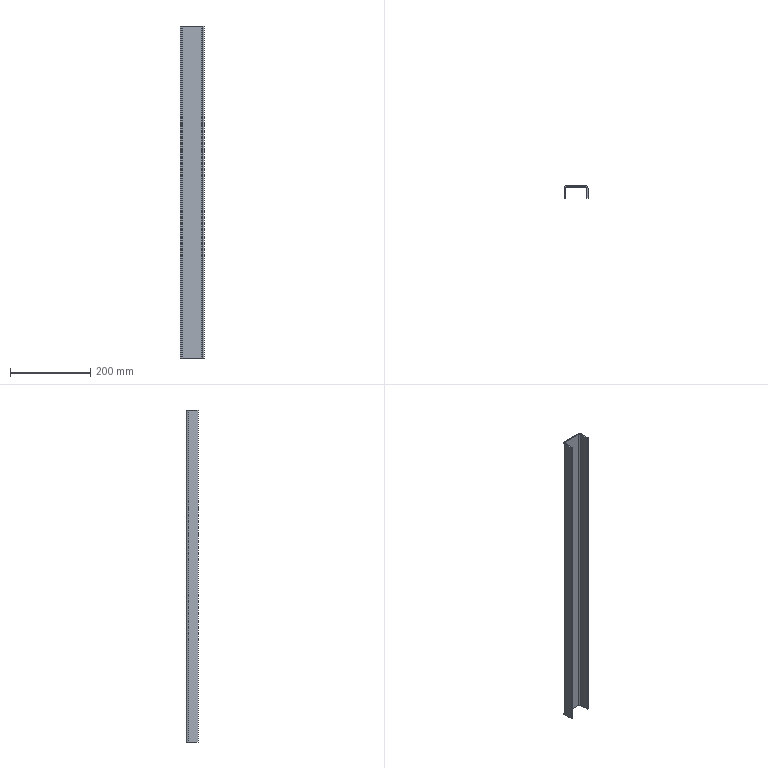Part | STEP file | VD-SYL0380DJ1006_1_1-13_VD-SYL0 | 1 solid | 14 faces | box 60 x 30 x 830 mm | volume 274242 mm3 | plane 10 | cylinder 4 | commonest cylinder face diameters 6 x2 12 x2
STEP:
#1=CARTESIAN_POINT('',(-24.,20.,415.));
#2=VERTEX_POINT('',#1);
#3=CARTESIAN_POINT('',(-24.,20.,-415.));
#4=VERTEX_POINT('',#3);
#5=CARTESIAN_POINT('',(-24.,20.,415.));
#6=DIRECTION('',(0.,0.,-1.));
#7=VECTOR('',#6,1000.);
#8=LINE('',#5,#7);
#9=EDGE_CURVE('',#2,#4,#8,.T.);
#10=ORIENTED_EDGE('',*,*,#9,.T.);
#11=CARTESIAN_POINT('',(-30.,14.,-415.));
#12=VERTEX_POINT('',#11);
#13=CARTESIAN_POINT('',(-24.,14.,-415.));
#14=DIRECTION('',(0.,0.,-1.));
#15=DIRECTION('',(-1.,0.,0.));
#16=AXIS2_PLACEMENT_3D('',#13,#14,#15);
#17=CIRCLE('',#16,6.);
#18=EDGE_CURVE('',#12,#4,#17,.T.);
#19=ORIENTED_EDGE('',*,*,#18,.F.);
#20=CARTESIAN_POINT('',(-30.,14.,415.));
#21=VERTEX_POINT('',#20);
#22=CARTESIAN_POINT('',(-30.,14.,-415.));
#23=DIRECTION('',(0.,0.,1.));
#24=VECTOR('',#23,1000.);
#25=LINE('',#22,#24);
#26=EDGE_CURVE('',#12,#21,#25,.T.);
#27=ORIENTED_EDGE('',*,*,#26,.T.);
#28=CARTESIAN_POINT('',(-24.,14.,415.));
#29=DIRECTION('',(0.,0.,1.));
#30=DIRECTION('',(0.,1.,0.));
#31=AXIS2_PLACEMENT_3D('',#28,#29,#30);
#32=CIRCLE('',#31,6.);
#33=EDGE_CURVE('',#2,#21,#32,.T.);
#34=ORIENTED_EDGE('',*,*,#33,.F.);
#35=EDGE_LOOP('',(#10,#19,#27,#34));
#36=FACE_OUTER_BOUND('',#35,.T.);
#37=CARTESIAN_POINT('',(-24.,14.,1496.988));
#38=DIRECTION('',(0.,0.,-1.));
#39=DIRECTION('',(-1.,0.,0.));
#40=AXIS2_PLACEMENT_3D('',#37,#38,#39);
#41=CYLINDRICAL_SURFACE('',#40,6.);
#42=ADVANCED_FACE('',(#36),#41,.T.);
#43=CARTESIAN_POINT('',(-30.,-10.,415.));
#44=VERTEX_POINT('',#43);
#45=CARTESIAN_POINT('',(-30.,-10.,-415.));
#46=VERTEX_POINT('',#45);
#47=CARTESIAN_POINT('',(-30.,-10.,415.));
#48=DIRECTION('',(0.,0.,-1.));
#49=VECTOR('',#48,1000.);
#50=LINE('',#47,#49);
#51=EDGE_CURVE('',#44,#46,#50,.T.);
#52=ORIENTED_EDGE('',*,*,#51,.T.);
#53=CARTESIAN_POINT('',(-27.,-10.,-415.));
#54=VERTEX_POINT('',#53);
#55=CARTESIAN_POINT('',(-27.,-10.,-415.));
#56=DIRECTION('',(-1.,0.,0.));
#57=VECTOR('',#56,1000.);
#58=LINE('',#55,#57);
#59=EDGE_CURVE('',#54,#46,#58,.T.);
#60=ORIENTED_EDGE('',*,*,#59,.F.);
#61=CARTESIAN_POINT('',(-27.,-10.,415.));
#62=VERTEX_POINT('',#61);
#63=CARTESIAN_POINT('',(-27.,-10.,415.));
#64=DIRECTION('',(0.,0.,-1.));
#65=VECTOR('',#64,1000.);
#66=LINE('',#63,#65);
#67=EDGE_CURVE('',#62,#54,#66,.T.);
#68=ORIENTED_EDGE('',*,*,#67,.F.);
#69=CARTESIAN_POINT('',(-30.,-10.,415.));
#70=DIRECTION('',(1.,0.,0.));
#71=VECTOR('',#70,1000.);
#72=LINE('',#69,#71);
#73=EDGE_CURVE('',#44,#62,#72,.T.);
#74=ORIENTED_EDGE('',*,*,#73,.F.);
#75=EDGE_LOOP('',(#52,#60,#68,#74));
#76=FACE_OUTER_BOUND('',#75,.T.);
#77=CARTESIAN_POINT('',(-28.5,-10.,0.));
#78=DIRECTION('',(0.,-1.,0.));
#79=DIRECTION('',(0.,0.,-1.));
#80=AXIS2_PLACEMENT_3D('',#77,#78,#79);
#81=PLANE('',#80);
#82=ADVANCED_FACE('',(#76),#81,.T.);
#83=CARTESIAN_POINT('',(-27.,14.,-415.));
#84=VERTEX_POINT('',#83);
#85=CARTESIAN_POINT('',(-27.,-10.,-415.));
#86=DIRECTION('',(0.,1.,0.));
#87=VECTOR('',#86,1000.);
#88=LINE('',#85,#87);
#89=EDGE_CURVE('',#54,#84,#88,.T.);
#90=ORIENTED_EDGE('',*,*,#89,.T.);
#91=CARTESIAN_POINT('',(-27.,14.,415.));
#92=VERTEX_POINT('',#91);
#93=CARTESIAN_POINT('',(-27.,14.,415.));
#94=DIRECTION('',(0.,0.,-1.));
#95=VECTOR('',#94,1000.);
#96=LINE('',#93,#95);
#97=EDGE_CURVE('',#92,#84,#96,.T.);
#98=ORIENTED_EDGE('',*,*,#97,.F.);
#99=CARTESIAN_POINT('',(-27.,-10.,415.));
#100=DIRECTION('',(0.,1.,0.));
#101=VECTOR('',#100,1000.);
#102=LINE('',#99,#101);
#103=EDGE_CURVE('',#62,#92,#102,.T.);
#104=ORIENTED_EDGE('',*,*,#103,.F.);
#105=ORIENTED_EDGE('',*,*,#67,.T.);
#106=EDGE_LOOP('',(#90,#98,#104,#105));
#107=FACE_OUTER_BOUND('',#106,.T.);
#108=CARTESIAN_POINT('',(-27.,20.,-415.));
#109=DIRECTION('',(-1.,0.,0.));
#110=DIRECTION('',(0.,0.,1.));
#111=AXIS2_PLACEMENT_3D('',#108,#109,#110);
#112=PLANE('',#111);
#113=ADVANCED_FACE('',(#107),#112,.F.);
#114=CARTESIAN_POINT('',(-24.,17.,-415.));
#115=VERTEX_POINT('',#114);
#116=CARTESIAN_POINT('',(-24.,14.,-415.));
#117=DIRECTION('',(0.,0.,1.));
#118=DIRECTION('',(0.,1.,0.));
#119=AXIS2_PLACEMENT_3D('',#116,#117,#118);
#120=CIRCLE('',#119,3.);
#121=EDGE_CURVE('',#115,#84,#120,.T.);
#122=ORIENTED_EDGE('',*,*,#121,.F.);
#123=CARTESIAN_POINT('',(-24.,17.,415.));
#124=VERTEX_POINT('',#123);
#125=CARTESIAN_POINT('',(-24.,17.,-415.));
#126=DIRECTION('',(0.,0.,1.));
#127=VECTOR('',#126,1000.);
#128=LINE('',#125,#127);
#129=EDGE_CURVE('',#115,#124,#128,.T.);
#130=ORIENTED_EDGE('',*,*,#129,.T.);
#131=CARTESIAN_POINT('',(-24.,14.,415.));
#132=DIRECTION('',(0.,0.,-1.));
#133=DIRECTION('',(-1.,0.,0.));
#134=AXIS2_PLACEMENT_3D('',#131,#132,#133);
#135=CIRCLE('',#134,3.);
#136=EDGE_CURVE('',#92,#124,#135,.T.);
#137=ORIENTED_EDGE('',*,*,#136,.F.);
#138=ORIENTED_EDGE('',*,*,#97,.T.);
#139=EDGE_LOOP('',(#122,#130,#137,#138));
#140=FACE_OUTER_BOUND('',#139,.T.);
#141=CARTESIAN_POINT('',(-24.,14.,1496.988));
#142=DIRECTION('',(0.,0.,-1.));
#143=DIRECTION('',(-1.,0.,0.));
#144=AXIS2_PLACEMENT_3D('',#141,#142,#143);
#145=CYLINDRICAL_SURFACE('',#144,3.);
#146=ADVANCED_FACE('',(#140),#145,.F.);
#147=CARTESIAN_POINT('',(30.,14.,415.));
#148=VERTEX_POINT('',#147);
#149=CARTESIAN_POINT('',(30.,14.,-415.));
#150=VERTEX_POINT('',#149);
#151=CARTESIAN_POINT('',(30.,14.,415.));
#152=DIRECTION('',(0.,0.,-1.));
#153=VECTOR('',#152,1000.);
#154=LINE('',#151,#153);
#155=EDGE_CURVE('',#148,#150,#154,.T.);
#156=ORIENTED_EDGE('',*,*,#155,.T.);
#157=CARTESIAN_POINT('',(24.,20.,-415.));
#158=VERTEX_POINT('',#157);
#159=CARTESIAN_POINT('',(24.,14.,-415.));
#160=DIRECTION('',(0.,0.,-1.));
#161=DIRECTION('',(0.,1.,0.));
#162=AXIS2_PLACEMENT_3D('',#159,#160,#161);
#163=CIRCLE('',#162,6.);
#164=EDGE_CURVE('',#158,#150,#163,.T.);
#165=ORIENTED_EDGE('',*,*,#164,.F.);
#166=CARTESIAN_POINT('',(24.,20.,415.));
#167=VERTEX_POINT('',#166);
#168=CARTESIAN_POINT('',(24.,20.,-415.));
#169=DIRECTION('',(0.,0.,1.));
#170=VECTOR('',#169,1000.);
#171=LINE('',#168,#170);
#172=EDGE_CURVE('',#158,#167,#171,.T.);
#173=ORIENTED_EDGE('',*,*,#172,.T.);
#174=CARTESIAN_POINT('',(24.,14.,415.));
#175=DIRECTION('',(0.,0.,1.));
#176=DIRECTION('',(1.,0.,0.));
#177=AXIS2_PLACEMENT_3D('',#174,#175,#176);
#178=CIRCLE('',#177,6.);
#179=EDGE_CURVE('',#148,#167,#178,.T.);
#180=ORIENTED_EDGE('',*,*,#179,.F.);
#181=EDGE_LOOP('',(#156,#165,#173,#180));
#182=FACE_OUTER_BOUND('',#181,.T.);
#183=CARTESIAN_POINT('',(24.,14.,1496.988));
#184=DIRECTION('',(0.,0.,-1.));
#185=DIRECTION('',(-1.,0.,0.));
#186=AXIS2_PLACEMENT_3D('',#183,#184,#185);
#187=CYLINDRICAL_SURFACE('',#186,6.);
#188=ADVANCED_FACE('',(#182),#187,.T.);
#189=ORIENTED_EDGE('',*,*,#155,.F.);
#190=CARTESIAN_POINT('',(30.,-10.,415.));
#191=VERTEX_POINT('',#190);
#192=CARTESIAN_POINT('',(30.,-10.,415.));
#193=DIRECTION('',(0.,1.,0.));
#194=VECTOR('',#193,1000.);
#195=LINE('',#192,#194);
#196=EDGE_CURVE('',#191,#148,#195,.T.);
#197=ORIENTED_EDGE('',*,*,#196,.F.);
#198=CARTESIAN_POINT('',(30.,-10.,-415.));
#199=VERTEX_POINT('',#198);
#200=CARTESIAN_POINT('',(30.,-10.,-415.));
#201=DIRECTION('',(0.,0.,1.));
#202=VECTOR('',#201,1000.);
#203=LINE('',#200,#202);
#204=EDGE_CURVE('',#199,#191,#203,.T.);
#205=ORIENTED_EDGE('',*,*,#204,.F.);
#206=CARTESIAN_POINT('',(30.,14.,-415.));
#207=DIRECTION('',(0.,-1.,0.));
#208=VECTOR('',#207,1000.);
#209=LINE('',#206,#208);
#210=EDGE_CURVE('',#150,#199,#209,.T.);
#211=ORIENTED_EDGE('',*,*,#210,.F.);
#212=EDGE_LOOP('',(#189,#197,#205,#211));
#213=FACE_OUTER_BOUND('',#212,.T.);
#214=CARTESIAN_POINT('',(30.,-10.,-415.));
#215=DIRECTION('',(1.,0.,0.));
#216=DIRECTION('',(0.,1.,0.));
#217=AXIS2_PLACEMENT_3D('',#214,#215,#216);
#218=PLANE('',#217);
#219=ADVANCED_FACE('',(#213),#218,.T.);
#220=CARTESIAN_POINT('',(27.,-10.,-415.));
#221=VERTEX_POINT('',#220);
#222=CARTESIAN_POINT('',(27.,-10.,-415.));
#223=DIRECTION('',(1.,0.,0.));
#224=VECTOR('',#223,1000.);
#225=LINE('',#222,#224);
#226=EDGE_CURVE('',#221,#199,#225,.T.);
#227=ORIENTED_EDGE('',*,*,#226,.T.);
#228=ORIENTED_EDGE('',*,*,#204,.T.);
#229=CARTESIAN_POINT('',(27.,-10.,415.));
#230=VERTEX_POINT('',#229);
#231=CARTESIAN_POINT('',(30.,-10.,415.));
#232=DIRECTION('',(-1.,0.,0.));
#233=VECTOR('',#232,1000.);
#234=LINE('',#231,#233);
#235=EDGE_CURVE('',#191,#230,#234,.T.);
#236=ORIENTED_EDGE('',*,*,#235,.T.);
#237=CARTESIAN_POINT('',(27.,-10.,415.));
#238=DIRECTION('',(0.,0.,-1.));
#239=VECTOR('',#238,1000.);
#240=LINE('',#237,#239);
#241=EDGE_CURVE('',#230,#221,#240,.T.);
#242=ORIENTED_EDGE('',*,*,#241,.T.);
#243=EDGE_LOOP('',(#227,#228,#236,#242));
#244=FACE_OUTER_BOUND('',#243,.T.);
#245=CARTESIAN_POINT('',(28.5,-10.,0.));
#246=DIRECTION('',(0.,1.,0.));
#247=DIRECTION('',(1.,0.,0.));
#248=AXIS2_PLACEMENT_3D('',#245,#246,#247);
#249=PLANE('',#248);
#250=ADVANCED_FACE('',(#244),#249,.F.);
#251=CARTESIAN_POINT('',(27.,14.,415.));
#252=VERTEX_POINT('',#251);
#253=CARTESIAN_POINT('',(27.,14.,415.));
#254=DIRECTION('',(0.,-1.,0.));
#255=VECTOR('',#254,1000.);
#256=LINE('',#253,#255);
#257=EDGE_CURVE('',#252,#230,#256,.T.);
#258=ORIENTED_EDGE('',*,*,#257,.F.);
#259=CARTESIAN_POINT('',(27.,14.,-415.));
#260=VERTEX_POINT('',#259);
#261=CARTESIAN_POINT('',(27.,14.,-415.));
#262=DIRECTION('',(0.,0.,1.));
#263=VECTOR('',#262,1000.);
#264=LINE('',#261,#263);
#265=EDGE_CURVE('',#260,#252,#264,.T.);
#266=ORIENTED_EDGE('',*,*,#265,.F.);
#267=CARTESIAN_POINT('',(27.,14.,-415.));
#268=DIRECTION('',(0.,-1.,0.));
#269=VECTOR('',#268,1000.);
#270=LINE('',#267,#269);
#271=EDGE_CURVE('',#260,#221,#270,.T.);
#272=ORIENTED_EDGE('',*,*,#271,.T.);
#273=ORIENTED_EDGE('',*,*,#241,.F.);
#274=EDGE_LOOP('',(#258,#266,#272,#273));
#275=FACE_OUTER_BOUND('',#274,.T.);
#276=CARTESIAN_POINT('',(27.,-10.,-415.));
#277=DIRECTION('',(1.,0.,0.));
#278=DIRECTION('',(0.,1.,0.));
#279=AXIS2_PLACEMENT_3D('',#276,#277,#278);
#280=PLANE('',#279);
#281=ADVANCED_FACE('',(#275),#280,.F.);
#282=CARTESIAN_POINT('',(24.,17.,-415.));
#283=VERTEX_POINT('',#282);
#284=CARTESIAN_POINT('',(24.,14.,-415.));
#285=DIRECTION('',(0.,0.,1.));
#286=DIRECTION('',(1.,0.,0.));
#287=AXIS2_PLACEMENT_3D('',#284,#285,#286);
#288=CIRCLE('',#287,3.);
#289=EDGE_CURVE('',#260,#283,#288,.T.);
#290=ORIENTED_EDGE('',*,*,#289,.F.);
#291=ORIENTED_EDGE('',*,*,#265,.T.);
#292=CARTESIAN_POINT('',(24.,17.,415.));
#293=VERTEX_POINT('',#292);
#294=CARTESIAN_POINT('',(24.,14.,415.));
#295=DIRECTION('',(0.,0.,-1.));
#296=DIRECTION('',(0.,1.,0.));
#297=AXIS2_PLACEMENT_3D('',#294,#295,#296);
#298=CIRCLE('',#297,3.);
#299=EDGE_CURVE('',#293,#252,#298,.T.);
#300=ORIENTED_EDGE('',*,*,#299,.F.);
#301=CARTESIAN_POINT('',(24.,17.,415.));
#302=DIRECTION('',(0.,0.,-1.));
#303=VECTOR('',#302,1000.);
#304=LINE('',#301,#303);
#305=EDGE_CURVE('',#293,#283,#304,.T.);
#306=ORIENTED_EDGE('',*,*,#305,.T.);
#307=EDGE_LOOP('',(#290,#291,#300,#306));
#308=FACE_OUTER_BOUND('',#307,.T.);
#309=CARTESIAN_POINT('',(24.,14.,1496.988));
#310=DIRECTION('',(0.,0.,-1.));
#311=DIRECTION('',(-1.,0.,0.));
#312=AXIS2_PLACEMENT_3D('',#309,#310,#311);
#313=CYLINDRICAL_SURFACE('',#312,3.);
#314=ADVANCED_FACE('',(#308),#313,.F.);
#315=CARTESIAN_POINT('',(-24.,17.,415.));
#316=DIRECTION('',(1.,0.,0.));
#317=VECTOR('',#316,1000.);
#318=LINE('',#315,#317);
#319=EDGE_CURVE('',#124,#293,#318,.T.);
#320=ORIENTED_EDGE('',*,*,#319,.F.);
#321=ORIENTED_EDGE('',*,*,#129,.F.);
#322=CARTESIAN_POINT('',(-24.,17.,-415.));
#323=DIRECTION('',(1.,0.,0.));
#324=VECTOR('',#323,1000.);
#325=LINE('',#322,#324);
#326=EDGE_CURVE('',#115,#283,#325,.T.);
#327=ORIENTED_EDGE('',*,*,#326,.T.);
#328=ORIENTED_EDGE('',*,*,#305,.F.);
#329=EDGE_LOOP('',(#320,#321,#327,#328));
#330=FACE_OUTER_BOUND('',#329,.T.);
#331=CARTESIAN_POINT('',(30.,17.,-415.));
#332=DIRECTION('',(0.,1.,0.));
#333=DIRECTION('',(1.,0.,0.));
#334=AXIS2_PLACEMENT_3D('',#331,#332,#333);
#335=PLANE('',#334);
#336=ADVANCED_FACE('',(#330),#335,.F.);
#337=ORIENTED_EDGE('',*,*,#121,.T.);
#338=ORIENTED_EDGE('',*,*,#89,.F.);
#339=ORIENTED_EDGE('',*,*,#59,.T.);
#340=CARTESIAN_POINT('',(-30.,-10.,-415.));
#341=DIRECTION('',(0.,1.,0.));
#342=VECTOR('',#341,1000.);
#343=LINE('',#340,#342);
#344=EDGE_CURVE('',#46,#12,#343,.T.);
#345=ORIENTED_EDGE('',*,*,#344,.T.);
#346=ORIENTED_EDGE('',*,*,#18,.T.);
#347=CARTESIAN_POINT('',(-24.,20.,-415.));
#348=DIRECTION('',(1.,0.,0.));
#349=VECTOR('',#348,1000.);
#350=LINE('',#347,#349);
#351=EDGE_CURVE('',#4,#158,#350,.T.);
#352=ORIENTED_EDGE('',*,*,#351,.T.);
#353=ORIENTED_EDGE('',*,*,#164,.T.);
#354=ORIENTED_EDGE('',*,*,#210,.T.);
#355=ORIENTED_EDGE('',*,*,#226,.F.);
#356=ORIENTED_EDGE('',*,*,#271,.F.);
#357=ORIENTED_EDGE('',*,*,#289,.T.);
#358=ORIENTED_EDGE('',*,*,#326,.F.);
#359=EDGE_LOOP('',(#337,#338,#339,#345,#346,#352,#353,#354,#355,#356,#357,#358));
#360=FACE_OUTER_BOUND('',#359,.T.);
#361=CARTESIAN_POINT('',(0.,18.5,-415.));
#362=DIRECTION('',(0.,0.,-1.));
#363=DIRECTION('',(0.,-1.,0.));
#364=AXIS2_PLACEMENT_3D('',#361,#362,#363);
#365=PLANE('',#364);
#366=ADVANCED_FACE('',(#360),#365,.T.);
#367=ORIENTED_EDGE('',*,*,#9,.F.);
#368=CARTESIAN_POINT('',(24.,20.,415.));
#369=DIRECTION('',(-1.,0.,0.));
#370=VECTOR('',#369,1000.);
#371=LINE('',#368,#370);
#372=EDGE_CURVE('',#167,#2,#371,.T.);
#373=ORIENTED_EDGE('',*,*,#372,.F.);
#374=ORIENTED_EDGE('',*,*,#172,.F.);
#375=ORIENTED_EDGE('',*,*,#351,.F.);
#376=EDGE_LOOP('',(#367,#373,#374,#375));
#377=FACE_OUTER_BOUND('',#376,.T.);
#378=CARTESIAN_POINT('',(30.,20.,-415.));
#379=DIRECTION('',(0.,1.,0.));
#380=DIRECTION('',(1.,0.,0.));
#381=AXIS2_PLACEMENT_3D('',#378,#379,#380);
#382=PLANE('',#381);
#383=ADVANCED_FACE('',(#377),#382,.T.);
#384=ORIENTED_EDGE('',*,*,#33,.T.);
#385=CARTESIAN_POINT('',(-30.,14.,415.));
#386=DIRECTION('',(0.,-1.,0.));
#387=VECTOR('',#386,1000.);
#388=LINE('',#385,#387);
#389=EDGE_CURVE('',#21,#44,#388,.T.);
#390=ORIENTED_EDGE('',*,*,#389,.T.);
#391=ORIENTED_EDGE('',*,*,#73,.T.);
#392=ORIENTED_EDGE('',*,*,#103,.T.);
#393=ORIENTED_EDGE('',*,*,#136,.T.);
#394=ORIENTED_EDGE('',*,*,#319,.T.);
#395=ORIENTED_EDGE('',*,*,#299,.T.);
#396=ORIENTED_EDGE('',*,*,#257,.T.);
#397=ORIENTED_EDGE('',*,*,#235,.F.);
#398=ORIENTED_EDGE('',*,*,#196,.T.);
#399=ORIENTED_EDGE('',*,*,#179,.T.);
#400=ORIENTED_EDGE('',*,*,#372,.T.);
#401=EDGE_LOOP('',(#384,#390,#391,#392,#393,#394,#395,#396,#397,#398,#399,#400));
#402=FACE_OUTER_BOUND('',#401,.T.);
#403=CARTESIAN_POINT('',(0.,18.5,415.));
#404=DIRECTION('',(0.,0.,-1.));
#405=DIRECTION('',(0.,-1.,0.));
#406=AXIS2_PLACEMENT_3D('',#403,#404,#405);
#407=PLANE('',#406);
#408=ADVANCED_FACE('',(#402),#407,.F.);
#409=ORIENTED_EDGE('',*,*,#26,.F.);
#410=ORIENTED_EDGE('',*,*,#344,.F.);
#411=ORIENTED_EDGE('',*,*,#51,.F.);
#412=ORIENTED_EDGE('',*,*,#389,.F.);
#413=EDGE_LOOP('',(#409,#410,#411,#412));
#414=FACE_OUTER_BOUND('',#413,.T.);
#415=CARTESIAN_POINT('',(-30.,20.,-415.));
#416=DIRECTION('',(-1.,0.,0.));
#417=DIRECTION('',(0.,0.,1.));
#418=AXIS2_PLACEMENT_3D('',#415,#416,#417);
#419=PLANE('',#418);
#420=ADVANCED_FACE('',(#414),#419,.T.);
#421=CLOSED_SHELL('',(#42,#82,#113,#146,#188,#219,#250,#281,#314,#336,#366,#383,#408,#420));
#422=MANIFOLD_SOLID_BREP('',#421);
#423=CARTESIAN_POINT('',(0.,0.,0.));
#424=DIRECTION('',(0.,0.,1.));
#425=DIRECTION('',(1.,0.,0.));
#426=AXIS2_PLACEMENT_3D('',#423,#424,#425);
#427=(LENGTH_UNIT()NAMED_UNIT(*)SI_UNIT(.MILLI.,.METRE.));
#428=UNCERTAINTY_MEASURE_WITH_UNIT(LENGTH_MEASURE(0.00001),#427,'','');
#429=(NAMED_UNIT(*)PLANE_ANGLE_UNIT()SI_UNIT($,.RADIAN.));
#430=(NAMED_UNIT(*)SI_UNIT($,.STERADIAN.)SOLID_ANGLE_UNIT());
#431=(GEOMETRIC_REPRESENTATION_CONTEXT(3)GLOBAL_UNCERTAINTY_ASSIGNED_CONTEXT((#428))GLOBAL_UNIT_ASSIGNED_CONTEXT((#427,#429,#430))REPRESENTATION_CONTEXT('',''));
#432=ADVANCED_BREP_SHAPE_REPRESENTATION('',(#422,#426),#431);